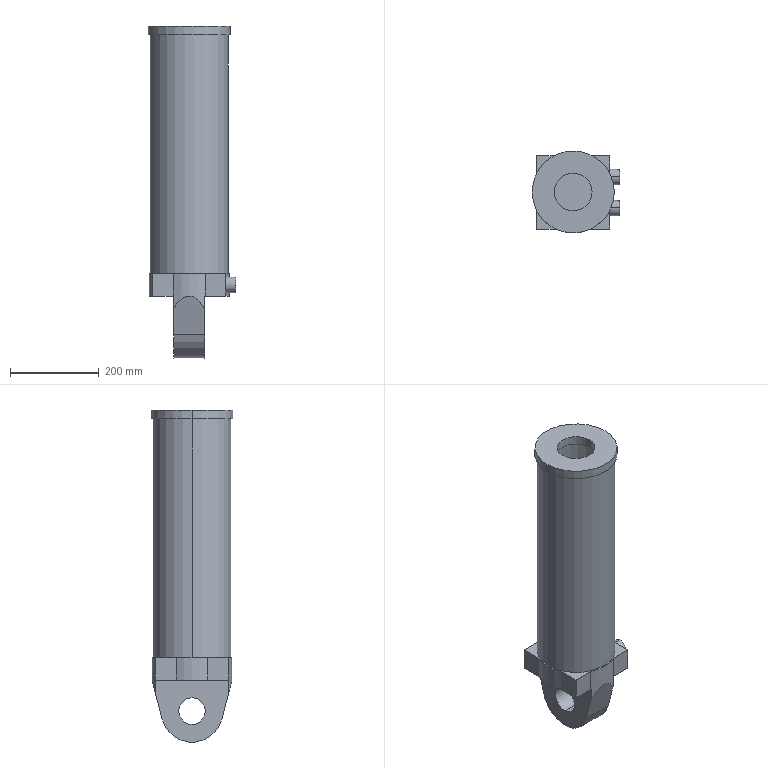Part | SolidWorks | features ICE 6, Extrusion 1 | 1 solid | 49 faces | box 197.5 x 185 x 748 mm | volume 5801023 mm3 | cylinder 26 | plane 23 | commonest cylinder face diameters 180 x7 25 x4 35 x4 60 x2 85 x2 155 x2